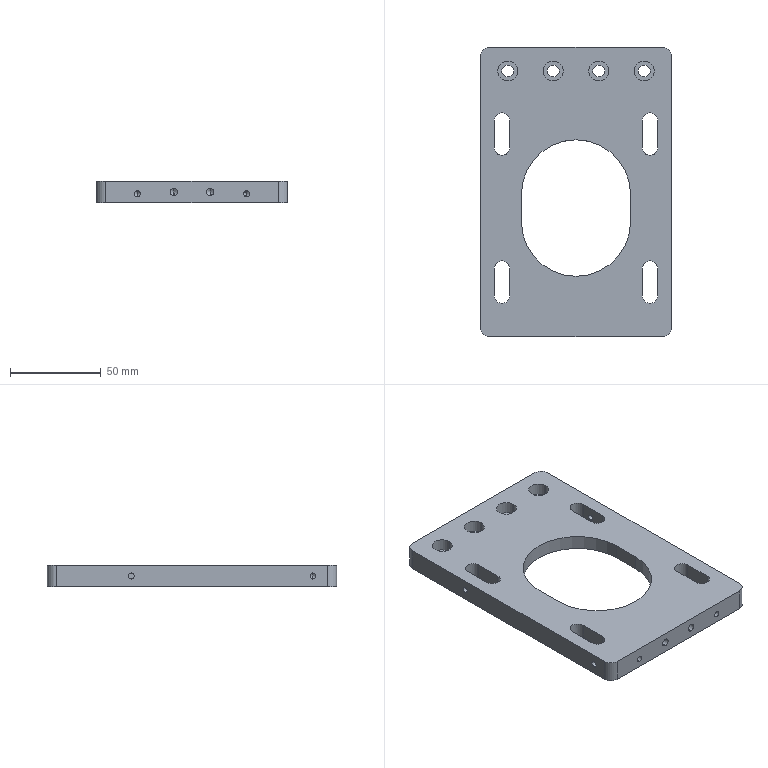Part | STEP file | 1 solid | 87 faces | box 105 x 159 x 12 mm | volume 123349 mm3 | cylinder 52 | plane 23 | cone 12 | commonest cylinder face diameters 3.3 x12 6.6 x8 8.5 x8 11 x8 95.5 x6 4.2 x4